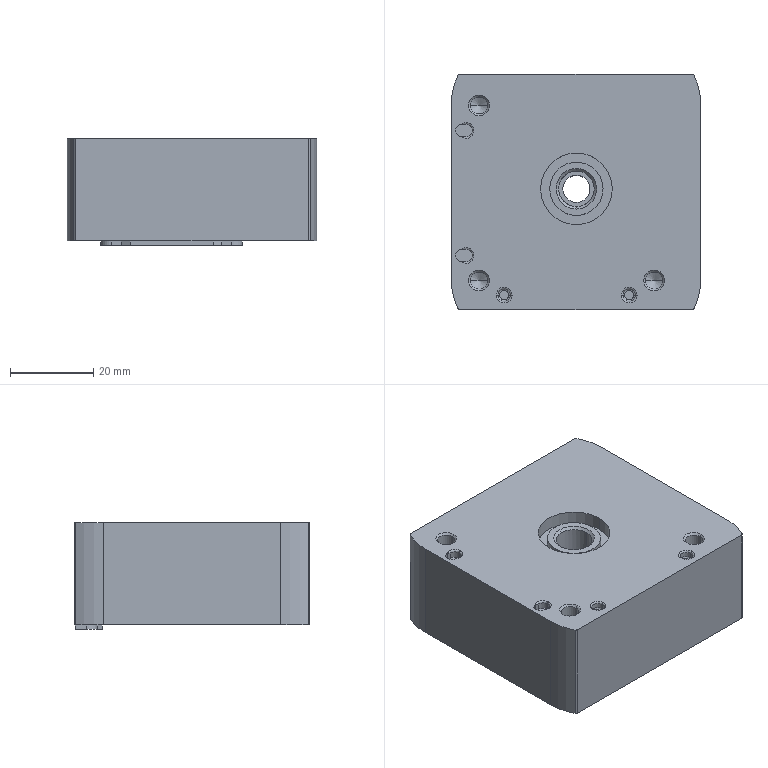Part | STEP file | DGC-25-G left fixed end | 1 solid | 125 faces | box 59.8 x 56.5 x 25.5 mm | volume 77572 mm3 | cylinder 54 | plane 43 | cone 16 | spline 12 | commonest cylinder face diameters 3 x10 5 x10 4.134 x6 6.5 x5 8.566 x5 1 x4